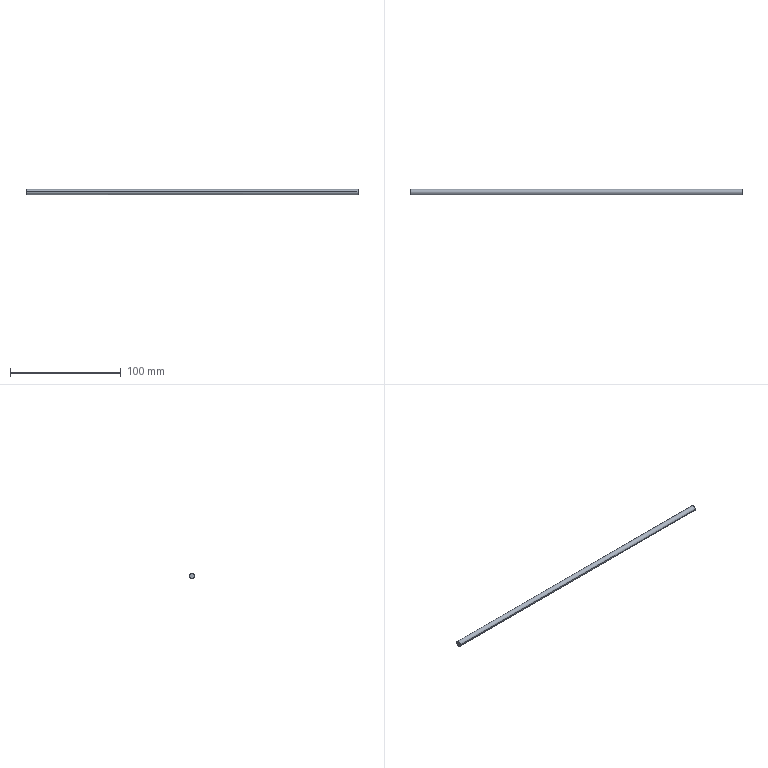Part | Creo | 1 solid | 4 faces | box 300 x 4.8 x 4.8 mm | volume 5429 mm3 | plane 2 | cylinder 2 | commonest cylinder face diameters 4.8 x2
STEP:
#1=CARTESIAN_POINT('',(370.,93.071,92.6));
#2=VERTEX_POINT('',#1);
#3=CARTESIAN_POINT('',(370.,95.471,95.));
#4=VERTEX_POINT('',#3);
#5=CARTESIAN_POINT('',(370.,93.071,95.));
#6=DIRECTION('',(1.,0.,0.));
#7=DIRECTION('',(0.,0.,-1.));
#8=AXIS2_PLACEMENT_3D('',#5,#6,#7);
#9=CIRCLE('',#8,2.4);
#10=EDGE_CURVE('',#2,#4,#9,.T.);
#11=ORIENTED_EDGE('',*,*,#10,.F.);
#12=CARTESIAN_POINT('',(370.,90.671,95.));
#13=VERTEX_POINT('',#12);
#14=CARTESIAN_POINT('',(370.,93.071,95.));
#15=DIRECTION('',(1.,0.,0.));
#16=DIRECTION('',(0.,-1.,0.));
#17=AXIS2_PLACEMENT_3D('',#14,#15,#16);
#18=CIRCLE('',#17,2.4);
#19=EDGE_CURVE('',#13,#2,#18,.T.);
#20=ORIENTED_EDGE('',*,*,#19,.F.);
#21=CARTESIAN_POINT('',(370.,93.071,95.));
#22=DIRECTION('',(1.,0.,0.));
#23=DIRECTION('',(0.,1.,0.));
#24=AXIS2_PLACEMENT_3D('',#21,#22,#23);
#25=CIRCLE('',#24,2.4);
#26=EDGE_CURVE('',#4,#13,#25,.T.);
#27=ORIENTED_EDGE('',*,*,#26,.F.);
#28=EDGE_LOOP('',(#11,#20,#27));
#29=FACE_OUTER_BOUND('',#28,.F.);
#30=CARTESIAN_POINT('',(370.,93.071,95.));
#31=DIRECTION('',(1.,0.,0.));
#32=DIRECTION('',(0.,0.,-1.));
#33=AXIS2_PLACEMENT_3D('',#30,#31,#32);
#34=PLANE('',#33);
#35=ADVANCED_FACE('',(#29),#34,.T.);
#36=CARTESIAN_POINT('',(70.,95.471,95.));
#37=VERTEX_POINT('',#36);
#38=CARTESIAN_POINT('',(70.,90.671,95.));
#39=VERTEX_POINT('',#38);
#40=CARTESIAN_POINT('',(70.,93.071,95.));
#41=DIRECTION('',(-1.,0.,0.));
#42=DIRECTION('',(0.,1.,0.));
#43=AXIS2_PLACEMENT_3D('',#40,#41,#42);
#44=CIRCLE('',#43,2.4);
#45=EDGE_CURVE('',#37,#39,#44,.T.);
#46=ORIENTED_EDGE('',*,*,#45,.T.);
#47=CARTESIAN_POINT('',(370.,90.671,95.));
#48=DIRECTION('',(-1.,0.,0.));
#49=VECTOR('',#48,300.);
#50=LINE('',#47,#49);
#51=EDGE_CURVE('',#13,#39,#50,.T.);
#52=ORIENTED_EDGE('',*,*,#51,.F.);
#53=ORIENTED_EDGE('',*,*,#19,.T.);
#54=ORIENTED_EDGE('',*,*,#10,.T.);
#55=CARTESIAN_POINT('',(370.,95.471,95.));
#56=DIRECTION('',(-1.,0.,0.));
#57=VECTOR('',#56,300.);
#58=LINE('',#55,#57);
#59=EDGE_CURVE('',#4,#37,#58,.T.);
#60=ORIENTED_EDGE('',*,*,#59,.T.);
#61=EDGE_LOOP('',(#46,#52,#53,#54,#60));
#62=FACE_OUTER_BOUND('',#61,.F.);
#63=CARTESIAN_POINT('',(120.,93.071,95.));
#64=DIRECTION('',(-1.,0.,0.));
#65=DIRECTION('',(0.,-1.,0.));
#66=AXIS2_PLACEMENT_3D('',#63,#64,#65);
#67=CYLINDRICAL_SURFACE('',#66,2.4);
#68=ADVANCED_FACE('',(#62),#67,.T.);
#69=ORIENTED_EDGE('',*,*,#45,.F.);
#70=CARTESIAN_POINT('',(70.,93.071,95.));
#71=DIRECTION('',(-1.,0.,0.));
#72=DIRECTION('',(0.,-1.,0.));
#73=AXIS2_PLACEMENT_3D('',#70,#71,#72);
#74=CIRCLE('',#73,2.4);
#75=EDGE_CURVE('',#39,#37,#74,.T.);
#76=ORIENTED_EDGE('',*,*,#75,.F.);
#77=EDGE_LOOP('',(#69,#76));
#78=FACE_OUTER_BOUND('',#77,.F.);
#79=CARTESIAN_POINT('',(70.,45.033,60.5));
#80=DIRECTION('',(1.,0.000000059,0.));
#81=DIRECTION('',(-0.000000059,1.,0.));
#82=AXIS2_PLACEMENT_3D('',#79,#80,#81);
#83=PLANE('',#82);
#84=ADVANCED_FACE('',(#78),#83,.F.);
#85=ORIENTED_EDGE('',*,*,#75,.T.);
#86=ORIENTED_EDGE('',*,*,#59,.F.);
#87=ORIENTED_EDGE('',*,*,#26,.T.);
#88=ORIENTED_EDGE('',*,*,#51,.T.);
#89=EDGE_LOOP('',(#85,#86,#87,#88));
#90=FACE_OUTER_BOUND('',#89,.F.);
#91=CARTESIAN_POINT('',(120.,93.071,95.));
#92=DIRECTION('',(-1.,0.,0.));
#93=DIRECTION('',(0.,-1.,0.));
#94=AXIS2_PLACEMENT_3D('',#91,#92,#93);
#95=CYLINDRICAL_SURFACE('',#94,2.4);
#96=ADVANCED_FACE('',(#90),#95,.T.);
#97=CLOSED_SHELL('',(#35,#68,#84,#96));
#98=MANIFOLD_SOLID_BREP('',#97);
#99=(LENGTH_UNIT()NAMED_UNIT(*)SI_UNIT(.MILLI.,.METRE.));
#100=UNCERTAINTY_MEASURE_WITH_UNIT(LENGTH_MEASURE(0.03001),#99,'','');
#101=(NAMED_UNIT(*)PLANE_ANGLE_UNIT()SI_UNIT($,.RADIAN.));
#102=PLANE_ANGLE_MEASURE_WITH_UNIT(PLANE_ANGLE_MEASURE(0.01745),#101);
#103=(CONVERSION_BASED_UNIT('DEGREE',#102)NAMED_UNIT(*)PLANE_ANGLE_UNIT());
#104=(NAMED_UNIT(*)SI_UNIT($,.STERADIAN.)SOLID_ANGLE_UNIT());
#105=(GEOMETRIC_REPRESENTATION_CONTEXT(3)GLOBAL_UNCERTAINTY_ASSIGNED_CONTEXT((#100))GLOBAL_UNIT_ASSIGNED_CONTEXT((#99,#103,#104))REPRESENTATION_CONTEXT('',''));
#106=ADVANCED_BREP_SHAPE_REPRESENTATION('',(#98),#105);